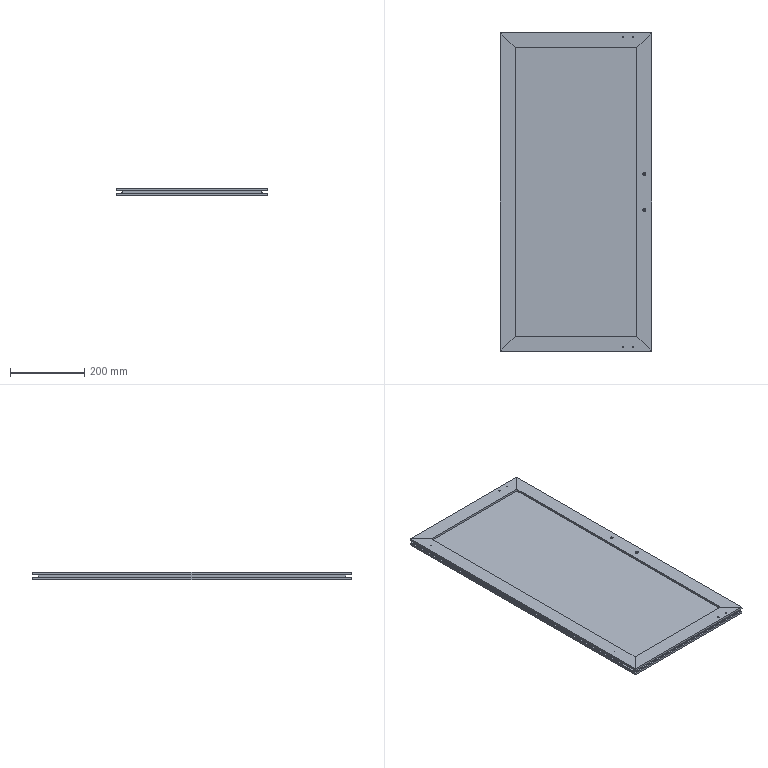Part | SolidWorks | features HoleWzd 3, ICE 1, WeldMemberFeat 1, WeldmentFeature 1 | 5 solids | 184 faces | box 407 x 856 x 20 mm | volume 2220771 mm3 | plane 132 | cylinder 44 | cone 8 | commonest cylinder face diameters 5 x16 3.3 x8 4.5 x8 6.5 x8 8 x4